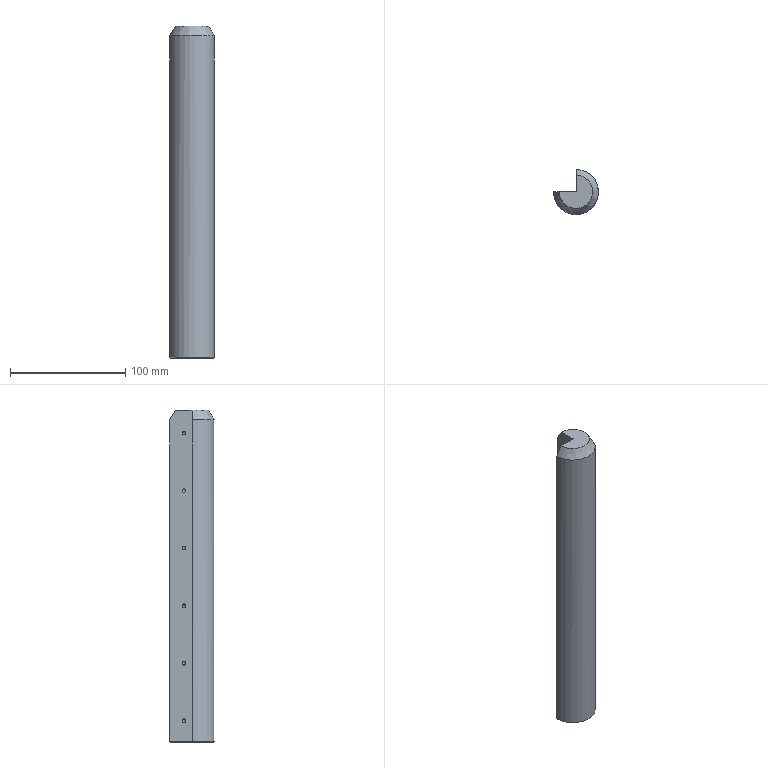Part | STEP file | Circlip fixture-medium storage post | 1 solid | 34 faces | box 39 x 38.994 x 288.5 mm | volume 253295 mm3 | cone 15 | cylinder 13 | plane 6 | commonest cylinder face diameters 3.3 x12 39 x1